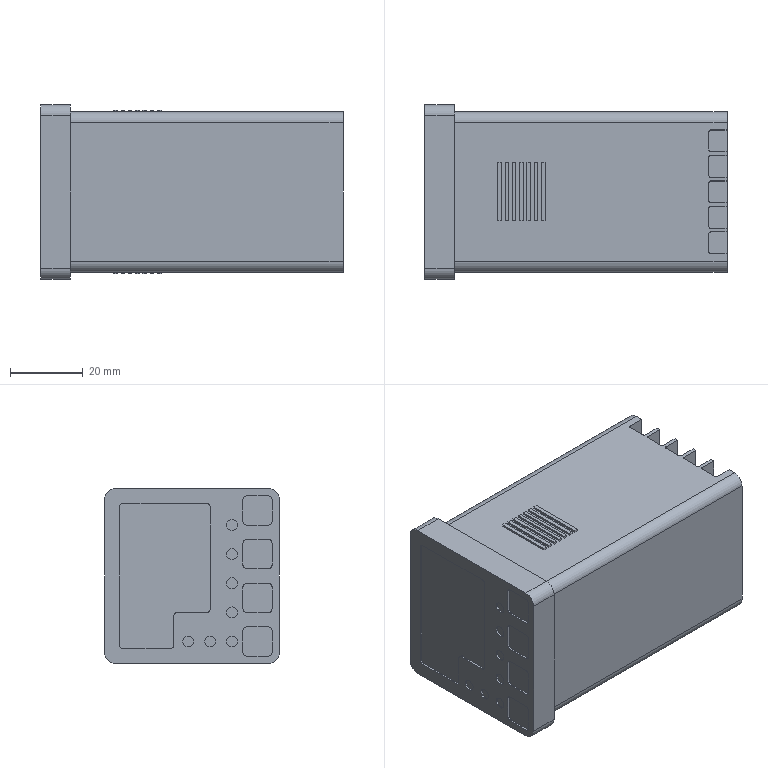Part | STEP file | Controller 2 | 1 solid | 219 faces | box 83 x 48 x 48 mm | volume 159214 mm3 | plane 155 | cylinder 64 | commonest cylinder face diameters 2 x22 1 x20 3 x14 6 x8